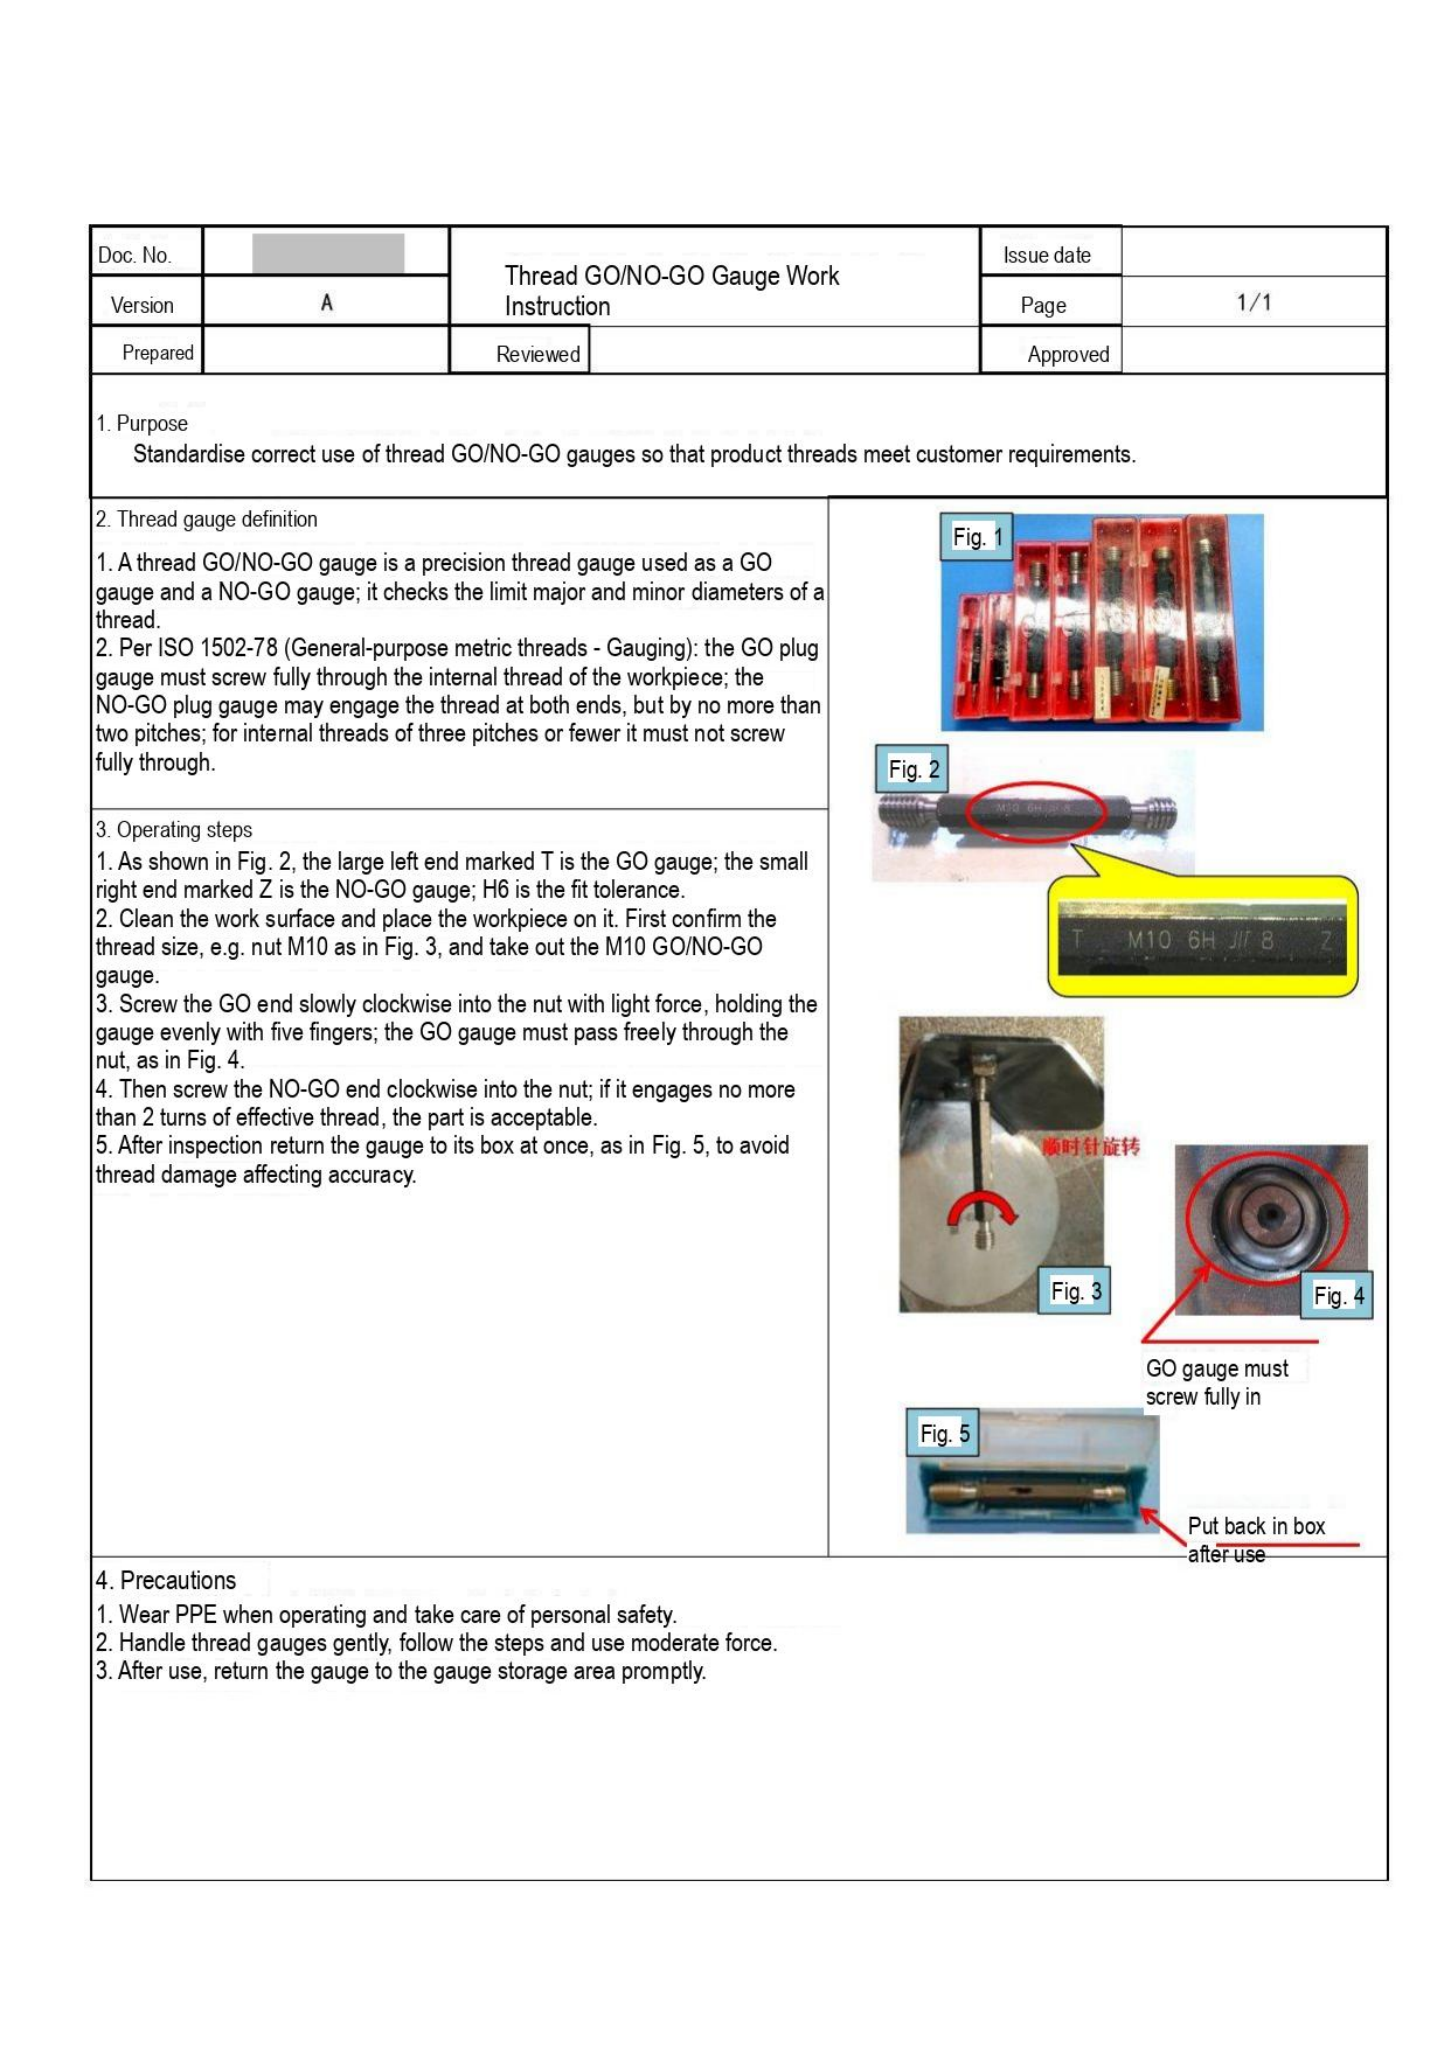| Doc. No. |  | Thread GO/NO-GO Gauge Work Instruction | Issue date |  |
|---|---|---|---|---|
| Version | A |  | Page | 1/1 |
| Prepared |  | Reviewed |  | Approved |

1. Purpose
Standardise correct use of thread GO/NO-GO gauges so that product threads meet customer requirements.

2. Thread gauge definition
1. A thread GO/NO-GO gauge is a precision thread gauge used as a GO gauge and a NO-GO gauge; it checks the limit major and minor diameters of a thread.
2. Per ISO 1502-78 (General-purpose metric threads - Gauging): the GO plug gauge must screw fully through the internal thread of the workpiece; the NO-GO plug gauge may engage the thread at both ends, but by no more than two pitches; for internal threads of three pitches or fewer it must not screw fully through.

Fig. 1

Fig. 2

T M10 6H J// 8 Z

3. Operating steps
1. As shown in Fig. 2, the large left end marked T is the GO gauge; the small right end marked Z is the NO-GO gauge; H6 is the fit tolerance.
2. Clean the work surface and place the workpiece on it. First confirm the thread size, e.g. nut M10 as in Fig. 3, and take out the M10 GO/NO-GO gauge.
3. Screw the GO end slowly clockwise into the nut with light force, holding the gauge evenly with five fingers; the GO gauge must pass freely through the nut, as in Fig. 4.
4. Then screw the NO-GO end clockwise into the nut; if it engages no more than 2 turns of effective thread, the part is acceptable.
5. After inspection return the gauge to its box at once, as in Fig. 5, to avoid thread damage affecting accuracy.

顺时针旋转

Fig. 3

Fig. 4

GO gauge must screw fully in

Fig. 5

Put back in box after use

4. Precautions
1. Wear PPE when operating and take care of personal safety.
2. Handle thread gauges gently, follow the steps and use moderate force.
3. After use, return the gauge to the gauge storage area promptly.